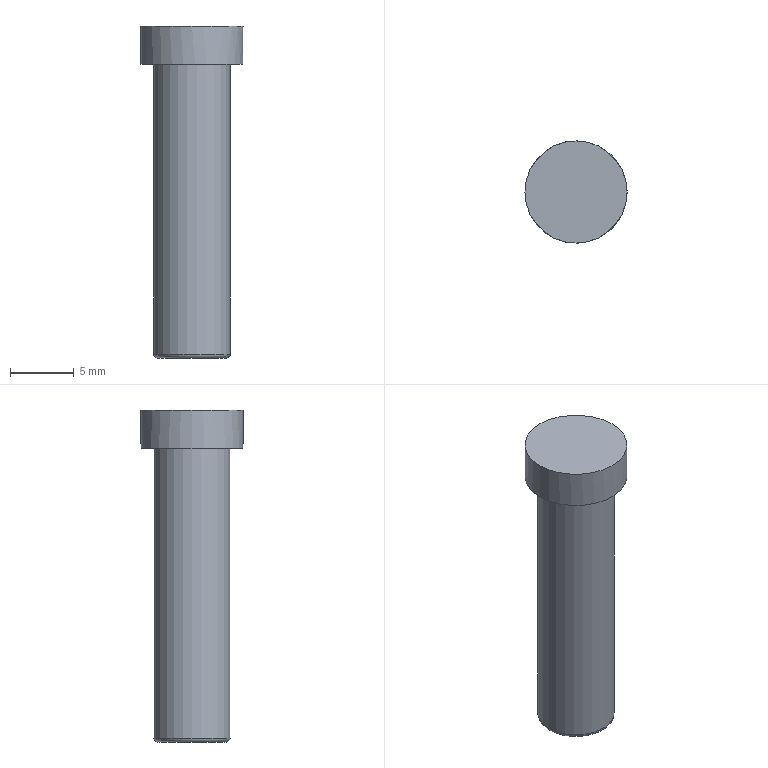Part | STEP file | gslz 2016.10.28-10_id3042_x_t | 1 solid | 6 faces | box 8 x 8 x 26 mm | volume 800.75 mm3 | plane 3 | cylinder 2 | torus 1 | commonest cylinder face diameters 6 x1 8 x1
STEP:
#1=CARTESIAN_POINT('',(0.,0.,0.));
#2=DIRECTION('',(0.,0.,1.));
#3=DIRECTION('',(1.,0.,0.));
#4=AXIS2_PLACEMENT_3D('',#1,#2,#3);
#5=CARTESIAN_POINT('',(-541.,163.,23.));
#6=VERTEX_POINT('',#5);
#7=CARTESIAN_POINT('',(-549.,163.,23.));
#8=VERTEX_POINT('',#7);
#9=CARTESIAN_POINT('',(-545.,163.,23.));
#10=DIRECTION('',(0.,0.,-1.));
#11=DIRECTION('',(1.,0.,0.));
#12=AXIS2_PLACEMENT_3D('',#9,#10,#11);
#13=CIRCLE('',#12,4.);
#14=CARTESIAN_POINT('',(-545.,163.,23.));
#15=DIRECTION('',(0.,0.,1.));
#16=DIRECTION('',(1.,0.,0.));
#17=AXIS2_PLACEMENT_3D('',#14,#15,#16);
#18=PLANE('',#17);
#19=CARTESIAN_POINT('',(4.,0.));
#20=CARTESIAN_POINT('',(4.,-6.928));
#21=CARTESIAN_POINT('',(-2.,-3.464));
#22=CARTESIAN_POINT('',(-8.,0.));
#23=CARTESIAN_POINT('',(-2.,3.464));
#24=CARTESIAN_POINT('',(4.,6.928));
#25=CARTESIAN_POINT('',(4.,0.));
#26=(BOUNDED_CURVE()B_SPLINE_CURVE(2,(#19,#20,#21,#22,#23,#24,#25),.UNSPECIFIED.,.T.,.F.)B_SPLINE_CURVE_WITH_KNOTS((1,2,2,2,2,1),(-2.094,0.,2.094,4.189,6.283,8.378),.UNSPECIFIED.)CURVE()GEOMETRIC_REPRESENTATION_ITEM()RATIONAL_B_SPLINE_CURVE((1.,0.5,1.,0.5,1.,0.5,1.))REPRESENTATION_ITEM(''));
#27=(GEOMETRIC_REPRESENTATION_CONTEXT(2)PARAMETRIC_REPRESENTATION_CONTEXT()REPRESENTATION_CONTEXT('',''));
#28=DEFINITIONAL_REPRESENTATION('',(#26),#27);
#29=PCURVE('',#18,#28);
#30=CARTESIAN_POINT('',(-545.,163.,23.));
#31=DIRECTION('',(0.,0.,-1.));
#32=DIRECTION('',(-1.,0.,0.));
#33=AXIS2_PLACEMENT_3D('',#30,#31,#32);
#34=CYLINDRICAL_SURFACE('',#33,4.);
#35=CARTESIAN_POINT('',(3.142,0.));
#36=DIRECTION('',(1.,0.));
#37=VECTOR('',#36,1.);
#38=LINE('',#35,#37);
#39=(GEOMETRIC_REPRESENTATION_CONTEXT(2)PARAMETRIC_REPRESENTATION_CONTEXT()REPRESENTATION_CONTEXT('',''));
#40=DEFINITIONAL_REPRESENTATION('',(#38),#39);
#41=PCURVE('',#34,#40);
#42=SURFACE_CURVE('',#13,(#29,#41),.PCURVE_S1.);
#43=EDGE_CURVE('',#6,#8,#42,.T.);
#44=ORIENTED_EDGE('',*,*,#43,.F.);
#45=CARTESIAN_POINT('',(-545.,163.,23.));
#46=DIRECTION('',(0.,0.,-1.));
#47=DIRECTION('',(1.,0.,0.));
#48=AXIS2_PLACEMENT_3D('',#45,#46,#47);
#49=CIRCLE('',#48,4.);
#50=CARTESIAN_POINT('',(4.,0.));
#51=CARTESIAN_POINT('',(4.,-6.928));
#52=CARTESIAN_POINT('',(-2.,-3.464));
#53=CARTESIAN_POINT('',(-8.,0.));
#54=CARTESIAN_POINT('',(-2.,3.464));
#55=CARTESIAN_POINT('',(4.,6.928));
#56=CARTESIAN_POINT('',(4.,0.));
#57=(BOUNDED_CURVE()B_SPLINE_CURVE(2,(#50,#51,#52,#53,#54,#55,#56),.UNSPECIFIED.,.T.,.F.)B_SPLINE_CURVE_WITH_KNOTS((1,2,2,2,2,1),(-2.094,0.,2.094,4.189,6.283,8.378),.UNSPECIFIED.)CURVE()GEOMETRIC_REPRESENTATION_ITEM()RATIONAL_B_SPLINE_CURVE((1.,0.5,1.,0.5,1.,0.5,1.))REPRESENTATION_ITEM(''));
#58=(GEOMETRIC_REPRESENTATION_CONTEXT(2)PARAMETRIC_REPRESENTATION_CONTEXT()REPRESENTATION_CONTEXT('',''));
#59=DEFINITIONAL_REPRESENTATION('',(#57),#58);
#60=PCURVE('',#18,#59);
#61=CARTESIAN_POINT('',(-3.142,0.));
#62=DIRECTION('',(1.,0.));
#63=VECTOR('',#62,1.);
#64=LINE('',#61,#63);
#65=(GEOMETRIC_REPRESENTATION_CONTEXT(2)PARAMETRIC_REPRESENTATION_CONTEXT()REPRESENTATION_CONTEXT('',''));
#66=DEFINITIONAL_REPRESENTATION('',(#64),#65);
#67=PCURVE('',#34,#66);
#68=SURFACE_CURVE('',#49,(#60,#67),.PCURVE_S1.);
#69=EDGE_CURVE('',#8,#6,#68,.T.);
#70=ORIENTED_EDGE('',*,*,#69,.F.);
#71=EDGE_LOOP('',(#44,#70));
#72=FACE_BOUND('',#71,.T.);
#73=ADVANCED_FACE('',(#72),#18,.T.);
#74=CARTESIAN_POINT('',(-548.,163.,20.));
#75=VERTEX_POINT('',#74);
#76=CARTESIAN_POINT('',(-545.,163.,20.));
#77=DIRECTION('',(0.,0.,-1.));
#78=DIRECTION('',(-1.,0.,0.));
#79=AXIS2_PLACEMENT_3D('',#76,#77,#78);
#80=CIRCLE('',#79,3.);
#81=CARTESIAN_POINT('',(-545.,163.,20.));
#82=DIRECTION('',(0.,0.,-1.));
#83=DIRECTION('',(-1.,0.,0.));
#84=AXIS2_PLACEMENT_3D('',#81,#82,#83);
#85=PLANE('',#84);
#86=CARTESIAN_POINT('',(0.,0.));
#87=DIRECTION('',(1.,0.));
#88=AXIS2_PLACEMENT_2D('',#86,#87);
#89=CIRCLE('',#88,3.);
#90=(GEOMETRIC_REPRESENTATION_CONTEXT(2)PARAMETRIC_REPRESENTATION_CONTEXT()REPRESENTATION_CONTEXT('',''));
#91=DEFINITIONAL_REPRESENTATION('',(#89),#90);
#92=PCURVE('',#85,#91);
#93=CARTESIAN_POINT('',(-545.,163.,19.));
#94=DIRECTION('',(0.,0.,-1.));
#95=DIRECTION('',(-1.,0.,0.));
#96=AXIS2_PLACEMENT_3D('',#93,#94,#95);
#97=CYLINDRICAL_SURFACE('',#96,3.);
#98=CARTESIAN_POINT('',(0.,-1.));
#99=DIRECTION('',(1.,0.));
#100=VECTOR('',#99,1.);
#101=LINE('',#98,#100);
#102=(GEOMETRIC_REPRESENTATION_CONTEXT(2)PARAMETRIC_REPRESENTATION_CONTEXT()REPRESENTATION_CONTEXT('',''));
#103=DEFINITIONAL_REPRESENTATION('',(#101),#102);
#104=PCURVE('',#97,#103);
#105=SURFACE_CURVE('',#80,(#92,#104),.PCURVE_S1.);
#106=EDGE_CURVE('',#75,#75,#105,.T.);
#107=ORIENTED_EDGE('',*,*,#106,.F.);
#108=EDGE_LOOP('',(#107));
#109=FACE_BOUND('',#108,.T.);
#110=CARTESIAN_POINT('',(-549.,163.,20.));
#111=VERTEX_POINT('',#110);
#112=CARTESIAN_POINT('',(-545.,163.,20.));
#113=DIRECTION('',(0.,0.,1.));
#114=DIRECTION('',(-1.,0.,0.));
#115=AXIS2_PLACEMENT_3D('',#112,#113,#114);
#116=CIRCLE('',#115,4.);
#117=CARTESIAN_POINT('',(4.,0.));
#118=CARTESIAN_POINT('',(4.,-6.928));
#119=CARTESIAN_POINT('',(-2.,-3.464));
#120=CARTESIAN_POINT('',(-8.,0.));
#121=CARTESIAN_POINT('',(-2.,3.464));
#122=CARTESIAN_POINT('',(4.,6.928));
#123=CARTESIAN_POINT('',(4.,0.));
#124=(BOUNDED_CURVE()B_SPLINE_CURVE(2,(#117,#118,#119,#120,#121,#122,#123),.UNSPECIFIED.,.T.,.F.)B_SPLINE_CURVE_WITH_KNOTS((1,2,2,2,2,1),(-2.094,0.,2.094,4.189,6.283,8.378),.UNSPECIFIED.)CURVE()GEOMETRIC_REPRESENTATION_ITEM()RATIONAL_B_SPLINE_CURVE((1.,0.5,1.,0.5,1.,0.5,1.))REPRESENTATION_ITEM(''));
#125=(GEOMETRIC_REPRESENTATION_CONTEXT(2)PARAMETRIC_REPRESENTATION_CONTEXT()REPRESENTATION_CONTEXT('',''));
#126=DEFINITIONAL_REPRESENTATION('',(#124),#125);
#127=PCURVE('',#85,#126);
#128=CARTESIAN_POINT('',(6.283,3.));
#129=DIRECTION('',(-1.,0.));
#130=VECTOR('',#129,1.);
#131=LINE('',#128,#130);
#132=(GEOMETRIC_REPRESENTATION_CONTEXT(2)PARAMETRIC_REPRESENTATION_CONTEXT()REPRESENTATION_CONTEXT('',''));
#133=DEFINITIONAL_REPRESENTATION('',(#131),#132);
#134=PCURVE('',#34,#133);
#135=SURFACE_CURVE('',#116,(#127,#134),.PCURVE_S1.);
#136=EDGE_CURVE('',#111,#111,#135,.T.);
#137=ORIENTED_EDGE('',*,*,#136,.F.);
#138=EDGE_LOOP('',(#137));
#139=FACE_BOUND('',#138,.T.);
#140=ADVANCED_FACE('',(#109,#139),#85,.T.);
#141=ORIENTED_EDGE('',*,*,#136,.T.);
#142=CARTESIAN_POINT('',(-549.,163.,23.));
#143=CARTESIAN_POINT('',(-549.,163.,20.));
#144=B_SPLINE_CURVE_WITH_KNOTS('',1,(#142,#143),.UNSPECIFIED.,.F.,.F.,(2,2),(0.,3.),.PIECEWISE_BEZIER_KNOTS.);
#145=CARTESIAN_POINT('',(0.,0.));
#146=DIRECTION('',(0.,1.));
#147=VECTOR('',#146,1.);
#148=LINE('',#145,#147);
#149=(GEOMETRIC_REPRESENTATION_CONTEXT(2)PARAMETRIC_REPRESENTATION_CONTEXT()REPRESENTATION_CONTEXT('',''));
#150=DEFINITIONAL_REPRESENTATION('',(#148),#149);
#151=PCURVE('',#34,#150);
#152=CARTESIAN_POINT('',(6.283,0.));
#153=DIRECTION('',(0.,1.));
#154=VECTOR('',#153,1.);
#155=LINE('',#152,#154);
#156=(GEOMETRIC_REPRESENTATION_CONTEXT(2)PARAMETRIC_REPRESENTATION_CONTEXT()REPRESENTATION_CONTEXT('',''));
#157=DEFINITIONAL_REPRESENTATION('',(#155),#156);
#158=PCURVE('',#34,#157);
#159=SEAM_CURVE('',#144,(#151,#158),.PCURVE_S1.);
#160=EDGE_CURVE('',#8,#111,#159,.T.);
#161=ORIENTED_EDGE('',*,*,#160,.F.);
#162=ORIENTED_EDGE('',*,*,#69,.T.);
#163=ORIENTED_EDGE('',*,*,#43,.T.);
#164=ORIENTED_EDGE('',*,*,#160,.T.);
#165=EDGE_LOOP('',(#141,#161,#162,#163,#164));
#166=FACE_BOUND('',#165,.T.);
#167=ADVANCED_FACE('',(#166),#34,.T.);
#168=CARTESIAN_POINT('',(-542.3,163.,-3.));
#169=VERTEX_POINT('',#168);
#170=CARTESIAN_POINT('',(-545.,163.,-3.));
#171=DIRECTION('',(0.,0.,-1.));
#172=DIRECTION('',(-1.,0.,0.));
#173=AXIS2_PLACEMENT_3D('',#170,#171,#172);
#174=CIRCLE('',#173,2.7);
#175=CARTESIAN_POINT('',(-545.,163.,-3.));
#176=DIRECTION('',(0.,0.,-1.));
#177=DIRECTION('',(-1.,0.,0.));
#178=AXIS2_PLACEMENT_3D('',#175,#176,#177);
#179=PLANE('',#178);
#180=CARTESIAN_POINT('',(0.,0.));
#181=DIRECTION('',(1.,0.));
#182=AXIS2_PLACEMENT_2D('',#180,#181);
#183=CIRCLE('',#182,2.7);
#184=(GEOMETRIC_REPRESENTATION_CONTEXT(2)PARAMETRIC_REPRESENTATION_CONTEXT()REPRESENTATION_CONTEXT('',''));
#185=DEFINITIONAL_REPRESENTATION('',(#183),#184);
#186=PCURVE('',#179,#185);
#187=CARTESIAN_POINT('',(-545.,163.,-2.7));
#188=DIRECTION('',(0.,0.,-1.));
#189=DIRECTION('',(1.,0.,0.));
#190=AXIS2_PLACEMENT_3D('',#187,#188,#189);
#191=TOROIDAL_SURFACE('',#190,2.7,0.3);
#192=CARTESIAN_POINT('',(-3.142,7.854));
#193=DIRECTION('',(1.,0.));
#194=VECTOR('',#193,1.);
#195=LINE('',#192,#194);
#196=(GEOMETRIC_REPRESENTATION_CONTEXT(2)PARAMETRIC_REPRESENTATION_CONTEXT()REPRESENTATION_CONTEXT('',''));
#197=DEFINITIONAL_REPRESENTATION('',(#195),#196);
#198=PCURVE('',#191,#197);
#199=SURFACE_CURVE('',#174,(#186,#198),.PCURVE_S1.);
#200=EDGE_CURVE('',#169,#169,#199,.T.);
#201=ORIENTED_EDGE('',*,*,#200,.T.);
#202=EDGE_LOOP('',(#201));
#203=FACE_BOUND('',#202,.T.);
#204=ADVANCED_FACE('',(#203),#179,.T.);
#205=CARTESIAN_POINT('',(-548.,163.,-2.7));
#206=VERTEX_POINT('',#205);
#207=CARTESIAN_POINT('',(-542.,163.,-2.7));
#208=VERTEX_POINT('',#207);
#209=CARTESIAN_POINT('',(-545.,163.,-2.7));
#210=DIRECTION('',(0.,0.,1.));
#211=DIRECTION('',(-1.,0.,0.));
#212=AXIS2_PLACEMENT_3D('',#209,#210,#211);
#213=CIRCLE('',#212,3.);
#214=CARTESIAN_POINT('',(6.283,21.7));
#215=DIRECTION('',(-1.,0.));
#216=VECTOR('',#215,1.);
#217=LINE('',#214,#216);
#218=(GEOMETRIC_REPRESENTATION_CONTEXT(2)PARAMETRIC_REPRESENTATION_CONTEXT()REPRESENTATION_CONTEXT('',''));
#219=DEFINITIONAL_REPRESENTATION('',(#217),#218);
#220=PCURVE('',#97,#219);
#221=CARTESIAN_POINT('',(3.142,6.283));
#222=DIRECTION('',(-1.,0.));
#223=VECTOR('',#222,1.);
#224=LINE('',#221,#223);
#225=(GEOMETRIC_REPRESENTATION_CONTEXT(2)PARAMETRIC_REPRESENTATION_CONTEXT()REPRESENTATION_CONTEXT('',''));
#226=DEFINITIONAL_REPRESENTATION('',(#224),#225);
#227=PCURVE('',#191,#226);
#228=SURFACE_CURVE('',#213,(#220,#227),.PCURVE_S1.);
#229=EDGE_CURVE('',#206,#208,#228,.T.);
#230=ORIENTED_EDGE('',*,*,#229,.T.);
#231=CARTESIAN_POINT('',(-545.,163.,-2.7));
#232=DIRECTION('',(0.,0.,1.));
#233=DIRECTION('',(-1.,0.,0.));
#234=AXIS2_PLACEMENT_3D('',#231,#232,#233);
#235=CIRCLE('',#234,3.);
#236=CARTESIAN_POINT('',(6.283,21.7));
#237=DIRECTION('',(-1.,0.));
#238=VECTOR('',#237,1.);
#239=LINE('',#236,#238);
#240=(GEOMETRIC_REPRESENTATION_CONTEXT(2)PARAMETRIC_REPRESENTATION_CONTEXT()REPRESENTATION_CONTEXT('',''));
#241=DEFINITIONAL_REPRESENTATION('',(#239),#240);
#242=PCURVE('',#97,#241);
#243=CARTESIAN_POINT('',(9.425,6.283));
#244=DIRECTION('',(-1.,0.));
#245=VECTOR('',#244,1.);
#246=LINE('',#243,#245);
#247=(GEOMETRIC_REPRESENTATION_CONTEXT(2)PARAMETRIC_REPRESENTATION_CONTEXT()REPRESENTATION_CONTEXT('',''));
#248=DEFINITIONAL_REPRESENTATION('',(#246),#247);
#249=PCURVE('',#191,#248);
#250=SURFACE_CURVE('',#235,(#242,#249),.PCURVE_S1.);
#251=EDGE_CURVE('',#208,#206,#250,.T.);
#252=ORIENTED_EDGE('',*,*,#251,.T.);
#253=CARTESIAN_POINT('',(-548.,163.,20.));
#254=CARTESIAN_POINT('',(-548.,163.,-2.7));
#255=B_SPLINE_CURVE_WITH_KNOTS('',1,(#253,#254),.UNSPECIFIED.,.F.,.F.,(2,2),(-1.,21.7),.PIECEWISE_BEZIER_KNOTS.);
#256=CARTESIAN_POINT('',(0.,0.));
#257=DIRECTION('',(0.,1.));
#258=VECTOR('',#257,1.);
#259=LINE('',#256,#258);
#260=(GEOMETRIC_REPRESENTATION_CONTEXT(2)PARAMETRIC_REPRESENTATION_CONTEXT()REPRESENTATION_CONTEXT('',''));
#261=DEFINITIONAL_REPRESENTATION('',(#259),#260);
#262=PCURVE('',#97,#261);
#263=CARTESIAN_POINT('',(6.283,0.));
#264=DIRECTION('',(0.,1.));
#265=VECTOR('',#264,1.);
#266=LINE('',#263,#265);
#267=(GEOMETRIC_REPRESENTATION_CONTEXT(2)PARAMETRIC_REPRESENTATION_CONTEXT()REPRESENTATION_CONTEXT('',''));
#268=DEFINITIONAL_REPRESENTATION('',(#266),#267);
#269=PCURVE('',#97,#268);
#270=SEAM_CURVE('',#255,(#262,#269),.PCURVE_S1.);
#271=EDGE_CURVE('',#75,#206,#270,.T.);
#272=ORIENTED_EDGE('',*,*,#271,.F.);
#273=ORIENTED_EDGE('',*,*,#106,.T.);
#274=ORIENTED_EDGE('',*,*,#271,.T.);
#275=EDGE_LOOP('',(#230,#252,#272,#273,#274));
#276=FACE_BOUND('',#275,.T.);
#277=ADVANCED_FACE('',(#276),#97,.T.);
#278=ORIENTED_EDGE('',*,*,#200,.F.);
#279=CARTESIAN_POINT('',(-542.,163.,-2.7));
#280=CARTESIAN_POINT('',(-542.,163.,-2.78));
#281=CARTESIAN_POINT('',(-542.026,163.,-2.858));
#282=CARTESIAN_POINT('',(-542.074,163.,-2.926));
#283=CARTESIAN_POINT('',(-542.142,163.,-2.974));
#284=CARTESIAN_POINT('',(-542.22,163.,-3.));
#285=CARTESIAN_POINT('',(-542.3,163.,-3.));
#286=(BOUNDED_CURVE()B_SPLINE_CURVE(6,(#279,#280,#281,#282,#283,#284,#285),.UNSPECIFIED.,.F.,.F.)B_SPLINE_CURVE_WITH_KNOTS((7,7),(0.,1.571),.PIECEWISE_BEZIER_KNOTS.)CURVE()GEOMETRIC_REPRESENTATION_ITEM()RATIONAL_B_SPLINE_CURVE((1.031,1.01,0.9979,0.994,0.9979,1.01,1.031))REPRESENTATION_ITEM(''));
#287=CARTESIAN_POINT('',(0.,6.283));
#288=DIRECTION('',(0.,1.));
#289=VECTOR('',#288,1.);
#290=LINE('',#287,#289);
#291=(GEOMETRIC_REPRESENTATION_CONTEXT(2)PARAMETRIC_REPRESENTATION_CONTEXT()REPRESENTATION_CONTEXT('',''));
#292=DEFINITIONAL_REPRESENTATION('',(#290),#291);
#293=PCURVE('',#191,#292);
#294=CARTESIAN_POINT('',(6.283,6.283));
#295=DIRECTION('',(0.,1.));
#296=VECTOR('',#295,1.);
#297=LINE('',#294,#296);
#298=(GEOMETRIC_REPRESENTATION_CONTEXT(2)PARAMETRIC_REPRESENTATION_CONTEXT()REPRESENTATION_CONTEXT('',''));
#299=DEFINITIONAL_REPRESENTATION('',(#297),#298);
#300=PCURVE('',#191,#299);
#301=SEAM_CURVE('',#286,(#293,#300),.PCURVE_S1.);
#302=EDGE_CURVE('',#208,#169,#301,.T.);
#303=ORIENTED_EDGE('',*,*,#302,.F.);
#304=ORIENTED_EDGE('',*,*,#229,.F.);
#305=ORIENTED_EDGE('',*,*,#251,.F.);
#306=ORIENTED_EDGE('',*,*,#302,.T.);
#307=EDGE_LOOP('',(#278,#303,#304,#305,#306));
#308=FACE_BOUND('',#307,.T.);
#309=ADVANCED_FACE('',(#308),#191,.T.);
#310=CLOSED_SHELL('',(#73,#140,#167,#204,#277,#309));
#311=MANIFOLD_SOLID_BREP('',#310);
#312=(LENGTH_UNIT()NAMED_UNIT(*)SI_UNIT(.MILLI.,.METRE.));
#313=UNCERTAINTY_MEASURE_WITH_UNIT(LENGTH_MEASURE(0.000005),#312,'','');
#314=(NAMED_UNIT(*)PLANE_ANGLE_UNIT()SI_UNIT($,.RADIAN.));
#315=(NAMED_UNIT(*)SI_UNIT($,.STERADIAN.)SOLID_ANGLE_UNIT());
#316=(GEOMETRIC_REPRESENTATION_CONTEXT(3)GLOBAL_UNCERTAINTY_ASSIGNED_CONTEXT((#313))GLOBAL_UNIT_ASSIGNED_CONTEXT((#312,#314,#315))REPRESENTATION_CONTEXT('',''));
#317=ADVANCED_BREP_SHAPE_REPRESENTATION('',(#4,#311),#316);